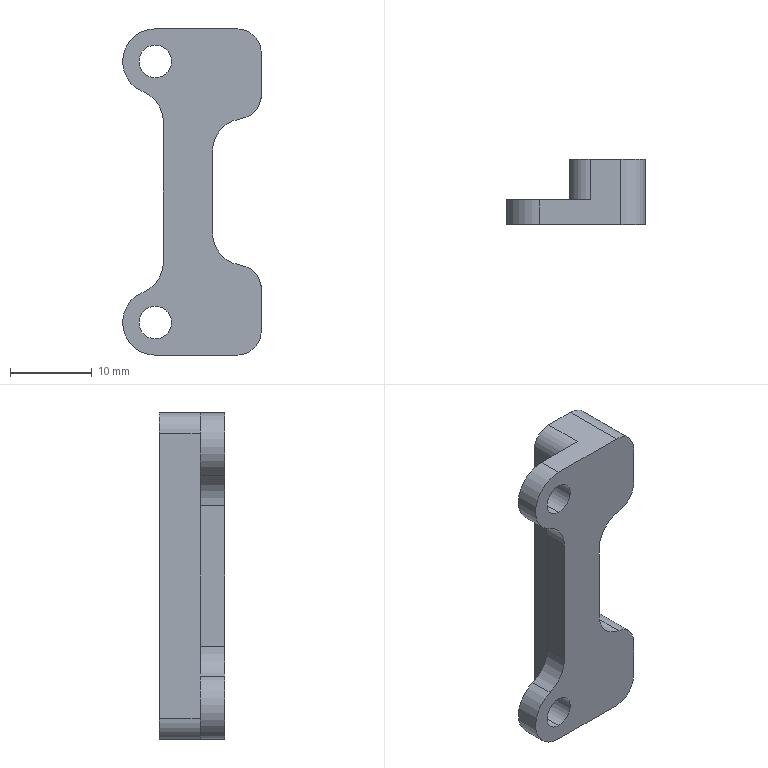CAM job | Mastercam | 3-axis milling, 5-axis milling, drilling | part box 17 x 8 x 40 mm | stock box 28 x 8 x 50 mm
Tools:
tool_number,name,type,diameter_mm,corner_radius_mm,flutes,flute_length_mm,overall_length_mm,shoulder_length_mm,holder_diameter_mm,length_offset,diameter_offset,default_rpm,default_feed_mm_min,default_plunge_mm_min,coolant
7,4 Chamfer Mill,chamfer mill,4,0,4,25,75,30,50,7,7,6250,750,600,COOL_OFF
8,8 Flat End Mill,end mill,8,0,4,25,75,25,50,8,8,1250,150,600,COOL_OFF
24,100 Flat End Mill,end mill,100,0,4,25,75,25,50,24,24,100,12,600,COOL_OFF
Operations:
seq,operation,operation_type,tool_number,tool_name,tool_diameter_mm,spindle_rpm,feed_mm_min,plunge_mm_min,retract_mm_min,cycle_time_s,wcs,posted,nc_file
1,Facing - [WCS: Plane] - [Tplane: Plane],Facing,24,100 Flat End Mill,100,4000,1000,600,1200,13.27,Plane,yes,.nc
2,2D High Speed (2D Dynamic Mill) - [WCS: Plane] - [Tplane: Plane],HighSpeed2D,8,8 Flat End Mill,8,7000,3000,600,1200,53.757,Plane,yes,.nc
3,Contour (Ramp) - [WCS: Plane] - [Tplane: Plane],Contour,8,8 Flat End Mill,8,7000,3000,600,1200,13.058,Plane,yes,.nc
4,Contour (2D) - [WCS: Plane] - [Tplane: Plane],Contour,8,8 Flat End Mill,8,7000,1000,600,1200,4.671,Plane,yes,.nc
5,Contour (2D) - [WCS: Plane] - [Tplane: Plane],Contour,8,8 Flat End Mill,8,7000,1000,600,1200,10.347,Plane,yes,.nc
6,Drill/Counterbore - [WCS: Plane] - [Tplane: Plane],Drill,7,4 Chamfer Mill,4,6000,200,600,1200,1.977,Plane,yes,.nc
7,Deburr 5-axis - [WCS: Plane] - [Tplane: Plane],459,7,4 Chamfer Mill,4,6000,1000,600,1200,13.321,Plane,yes,.nc